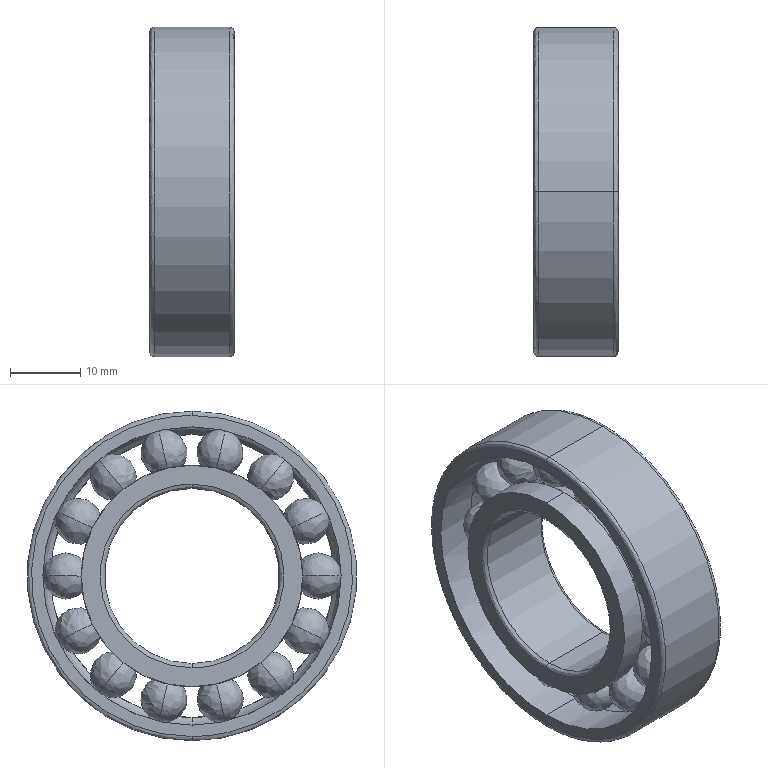Part | STEP file | 6005-2Z_1 | 1 solid | 82 faces | box 12 x 47 x 47 mm | volume 9163 mm3 | spline 66 | cylinder 12 | plane 4 | commonest cylinder face diameters 25 x2 29.45 x2 31.6 x2 40.4 x2 42.55 x2 47 x2